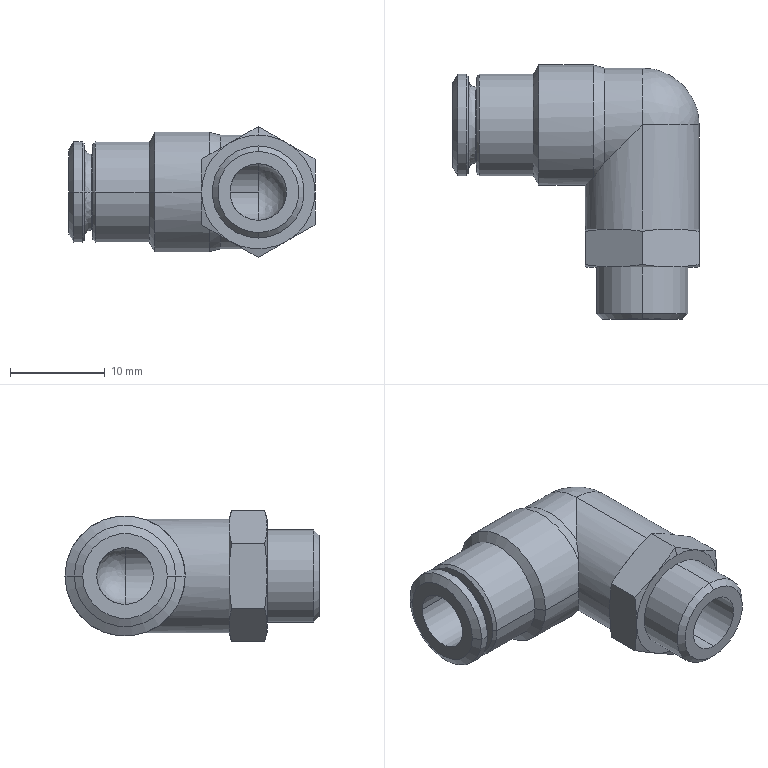Part | STEP file | PN62195-005_METRIC_PLASTIC_TUBE_FITTING | 1 solid | 57 faces | box 26 x 26.85 x 13.856 mm | volume 3050 mm3 | cone 24 | cylinder 18 | plane 11 | spline 4 | commonest cylinder face diameters 6 x4 10.7 x4 12 x4 8 x2 9.728 x2 12.7 x2